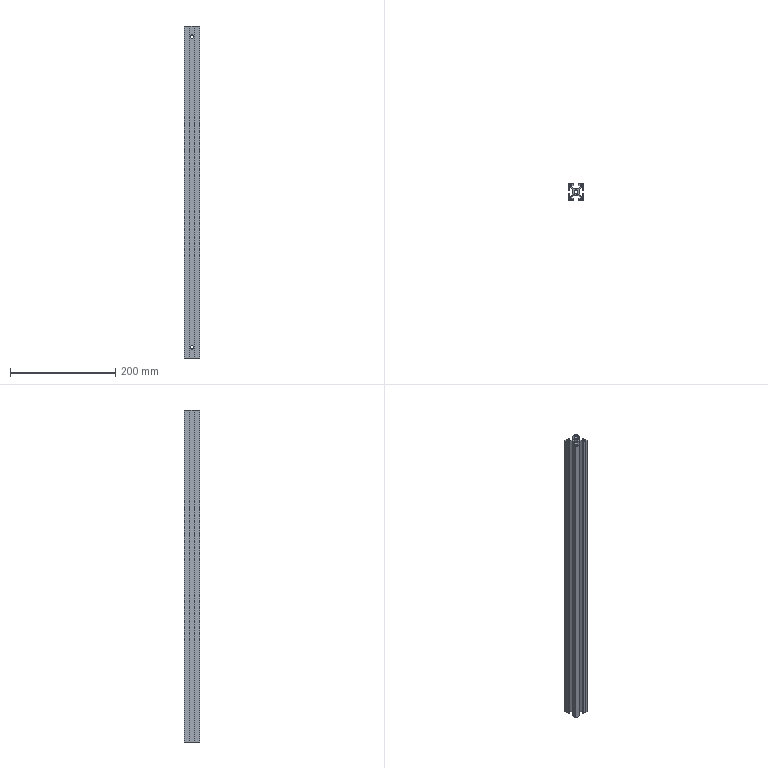Part | SolidWorks | features 3DProfileFeature 1, Extrusion 1, HoleWzd 1 | 1 solid | 192 faces | box 30 x 30.001 x 630 mm | volume 208708 mm3 | cylinder 102 | plane 90 | commonest cylinder face diameters 0.6 x72 2 x16 6.6 x8 11 x4 6.8 x2